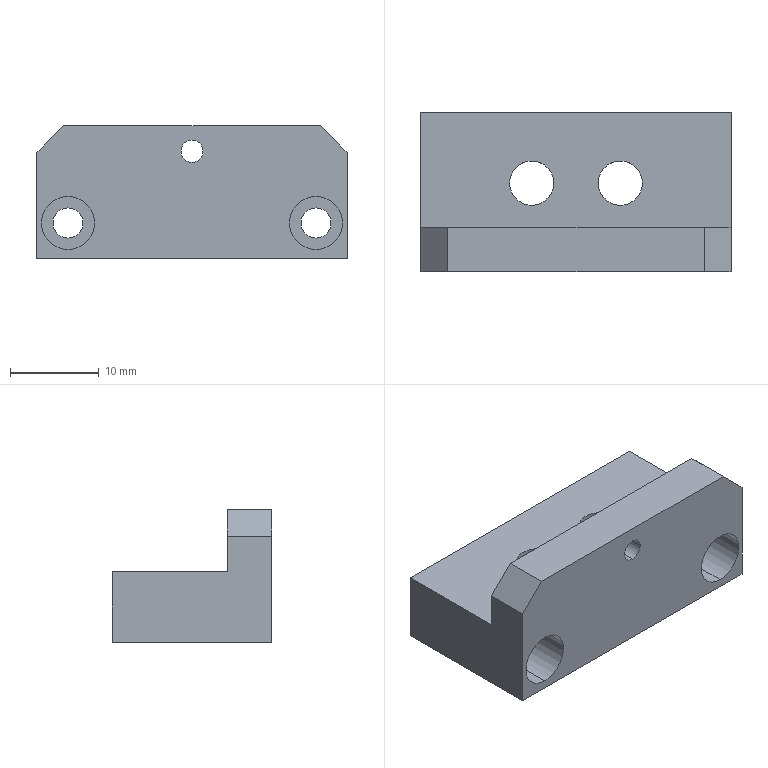Part | SolidWorks | features HoleWzd 4, Chamfer 1, Extrusion 1, ICE 1 | 1 solid | 34 faces | box 35 x 18 x 15 mm | volume 5316 mm3 | cylinder 18 | plane 12 | cone 4 | commonest cylinder face diameters 3 x4 3.4 x4 5 x4 6 x4 2.5 x2
STEP:
#1=CARTESIAN_POINT('',(-14.,-4.,-0.5));
#2=VERTEX_POINT('',#1);
#3=CARTESIAN_POINT('',(-14.,-4.,-6.5));
#4=VERTEX_POINT('',#3);
#5=CARTESIAN_POINT('',(-14.,-4.,-3.5));
#6=DIRECTION('',(0.,-1.,0.));
#7=DIRECTION('',(0.,0.,-1.));
#8=AXIS2_PLACEMENT_3D('',#5,#6,#7);
#9=CIRCLE('',#8,3.);
#10=EDGE_CURVE('',#2,#4,#9,.T.);
#11=ORIENTED_EDGE('',*,*,#10,.F.);
#12=CARTESIAN_POINT('',(-14.,-9.,-0.5));
#13=VERTEX_POINT('',#12);
#14=CARTESIAN_POINT('',(-14.,-9.,-0.5));
#15=DIRECTION('',(0.,-1.,0.));
#16=VECTOR('',#15,1000.);
#17=LINE('',#14,#16);
#18=EDGE_CURVE('',#2,#13,#17,.T.);
#19=ORIENTED_EDGE('',*,*,#18,.T.);
#20=CARTESIAN_POINT('',(-14.,-9.,-6.5));
#21=VERTEX_POINT('',#20);
#22=CARTESIAN_POINT('',(-14.,-9.,-3.5));
#23=DIRECTION('',(0.,-1.,0.));
#24=DIRECTION('',(0.,0.,-1.));
#25=AXIS2_PLACEMENT_3D('',#22,#23,#24);
#26=CIRCLE('',#25,3.);
#27=EDGE_CURVE('',#13,#21,#26,.T.);
#28=ORIENTED_EDGE('',*,*,#27,.T.);
#29=CARTESIAN_POINT('',(-14.,-9.,-6.5));
#30=DIRECTION('',(0.,-1.,0.));
#31=VECTOR('',#30,1000.);
#32=LINE('',#29,#31);
#33=EDGE_CURVE('',#4,#21,#32,.T.);
#34=ORIENTED_EDGE('',*,*,#33,.F.);
#35=EDGE_LOOP('',(#11,#19,#28,#34));
#36=FACE_OUTER_BOUND('',#35,.T.);
#37=CARTESIAN_POINT('',(-14.,-9.,-3.5));
#38=DIRECTION('',(0.,-1.,0.));
#39=DIRECTION('',(0.,0.,-1.));
#40=AXIS2_PLACEMENT_3D('',#37,#38,#39);
#41=CYLINDRICAL_SURFACE('',#40,3.);
#42=ADVANCED_FACE('',(#36),#41,.F.);
#43=CARTESIAN_POINT('',(-14.,9.,-1.8));
#44=VERTEX_POINT('',#43);
#45=CARTESIAN_POINT('',(-14.,9.,-5.2));
#46=VERTEX_POINT('',#45);
#47=CARTESIAN_POINT('',(-14.,9.,-3.5));
#48=DIRECTION('',(0.,-1.,0.));
#49=DIRECTION('',(0.,0.,-1.));
#50=AXIS2_PLACEMENT_3D('',#47,#48,#49);
#51=CIRCLE('',#50,1.7);
#52=EDGE_CURVE('',#44,#46,#51,.T.);
#53=ORIENTED_EDGE('',*,*,#52,.F.);
#54=CARTESIAN_POINT('',(-14.,-4.,-1.8));
#55=VERTEX_POINT('',#54);
#56=CARTESIAN_POINT('',(-14.,-9.,-1.8));
#57=DIRECTION('',(0.,-1.,0.));
#58=VECTOR('',#57,1000.);
#59=LINE('',#56,#58);
#60=EDGE_CURVE('',#44,#55,#59,.T.);
#61=ORIENTED_EDGE('',*,*,#60,.T.);
#62=CARTESIAN_POINT('',(-14.,-4.,-5.2));
#63=VERTEX_POINT('',#62);
#64=CARTESIAN_POINT('',(-14.,-4.,-3.5));
#65=DIRECTION('',(0.,-1.,0.));
#66=DIRECTION('',(0.,0.,-1.));
#67=AXIS2_PLACEMENT_3D('',#64,#65,#66);
#68=CIRCLE('',#67,1.7);
#69=EDGE_CURVE('',#55,#63,#68,.T.);
#70=ORIENTED_EDGE('',*,*,#69,.T.);
#71=CARTESIAN_POINT('',(-14.,-9.,-5.2));
#72=DIRECTION('',(0.,-1.,0.));
#73=VECTOR('',#72,1000.);
#74=LINE('',#71,#73);
#75=EDGE_CURVE('',#46,#63,#74,.T.);
#76=ORIENTED_EDGE('',*,*,#75,.F.);
#77=EDGE_LOOP('',(#53,#61,#70,#76));
#78=FACE_OUTER_BOUND('',#77,.T.);
#79=CARTESIAN_POINT('',(-14.,-9.,-3.5));
#80=DIRECTION('',(0.,-1.,0.));
#81=DIRECTION('',(0.,0.,-1.));
#82=AXIS2_PLACEMENT_3D('',#79,#80,#81);
#83=CYLINDRICAL_SURFACE('',#82,1.7);
#84=ADVANCED_FACE('',(#78),#83,.F.);
#85=CARTESIAN_POINT('',(14.,-4.,-0.5));
#86=VERTEX_POINT('',#85);
#87=CARTESIAN_POINT('',(14.,-4.,-6.5));
#88=VERTEX_POINT('',#87);
#89=CARTESIAN_POINT('',(14.,-4.,-3.5));
#90=DIRECTION('',(0.,-1.,0.));
#91=DIRECTION('',(0.,0.,-1.));
#92=AXIS2_PLACEMENT_3D('',#89,#90,#91);
#93=CIRCLE('',#92,3.);
#94=EDGE_CURVE('',#86,#88,#93,.T.);
#95=ORIENTED_EDGE('',*,*,#94,.F.);
#96=CARTESIAN_POINT('',(14.,-9.,-0.5));
#97=VERTEX_POINT('',#96);
#98=CARTESIAN_POINT('',(14.,-9.,-0.5));
#99=DIRECTION('',(0.,-1.,0.));
#100=VECTOR('',#99,1000.);
#101=LINE('',#98,#100);
#102=EDGE_CURVE('',#86,#97,#101,.T.);
#103=ORIENTED_EDGE('',*,*,#102,.T.);
#104=CARTESIAN_POINT('',(14.,-9.,-6.5));
#105=VERTEX_POINT('',#104);
#106=CARTESIAN_POINT('',(14.,-9.,-3.5));
#107=DIRECTION('',(0.,-1.,0.));
#108=DIRECTION('',(0.,0.,-1.));
#109=AXIS2_PLACEMENT_3D('',#106,#107,#108);
#110=CIRCLE('',#109,3.);
#111=EDGE_CURVE('',#97,#105,#110,.T.);
#112=ORIENTED_EDGE('',*,*,#111,.T.);
#113=CARTESIAN_POINT('',(14.,-9.,-6.5));
#114=DIRECTION('',(0.,-1.,0.));
#115=VECTOR('',#114,1000.);
#116=LINE('',#113,#115);
#117=EDGE_CURVE('',#88,#105,#116,.T.);
#118=ORIENTED_EDGE('',*,*,#117,.F.);
#119=EDGE_LOOP('',(#95,#103,#112,#118));
#120=FACE_OUTER_BOUND('',#119,.T.);
#121=CARTESIAN_POINT('',(14.,-9.,-3.5));
#122=DIRECTION('',(0.,-1.,0.));
#123=DIRECTION('',(0.,0.,-1.));
#124=AXIS2_PLACEMENT_3D('',#121,#122,#123);
#125=CYLINDRICAL_SURFACE('',#124,3.);
#126=ADVANCED_FACE('',(#120),#125,.F.);
#127=CARTESIAN_POINT('',(14.,9.,-1.8));
#128=VERTEX_POINT('',#127);
#129=CARTESIAN_POINT('',(14.,9.,-5.2));
#130=VERTEX_POINT('',#129);
#131=CARTESIAN_POINT('',(14.,9.,-3.5));
#132=DIRECTION('',(0.,-1.,0.));
#133=DIRECTION('',(0.,0.,-1.));
#134=AXIS2_PLACEMENT_3D('',#131,#132,#133);
#135=CIRCLE('',#134,1.7);
#136=EDGE_CURVE('',#128,#130,#135,.T.);
#137=ORIENTED_EDGE('',*,*,#136,.F.);
#138=CARTESIAN_POINT('',(14.,-4.,-1.8));
#139=VERTEX_POINT('',#138);
#140=CARTESIAN_POINT('',(14.,-9.,-1.8));
#141=DIRECTION('',(0.,-1.,0.));
#142=VECTOR('',#141,1000.);
#143=LINE('',#140,#142);
#144=EDGE_CURVE('',#128,#139,#143,.T.);
#145=ORIENTED_EDGE('',*,*,#144,.T.);
#146=CARTESIAN_POINT('',(14.,-4.,-5.2));
#147=VERTEX_POINT('',#146);
#148=CARTESIAN_POINT('',(14.,-4.,-3.5));
#149=DIRECTION('',(0.,-1.,0.));
#150=DIRECTION('',(0.,0.,-1.));
#151=AXIS2_PLACEMENT_3D('',#148,#149,#150);
#152=CIRCLE('',#151,1.7);
#153=EDGE_CURVE('',#139,#147,#152,.T.);
#154=ORIENTED_EDGE('',*,*,#153,.T.);
#155=CARTESIAN_POINT('',(14.,-9.,-5.2));
#156=DIRECTION('',(0.,-1.,0.));
#157=VECTOR('',#156,1000.);
#158=LINE('',#155,#157);
#159=EDGE_CURVE('',#130,#147,#158,.T.);
#160=ORIENTED_EDGE('',*,*,#159,.F.);
#161=EDGE_LOOP('',(#137,#145,#154,#160));
#162=FACE_OUTER_BOUND('',#161,.T.);
#163=CARTESIAN_POINT('',(14.,-9.,-3.5));
#164=DIRECTION('',(0.,-1.,0.));
#165=DIRECTION('',(0.,0.,-1.));
#166=AXIS2_PLACEMENT_3D('',#163,#164,#165);
#167=CYLINDRICAL_SURFACE('',#166,1.7);
#168=ADVANCED_FACE('',(#162),#167,.F.);
#169=CARTESIAN_POINT('',(0.,-4.,5.85));
#170=VERTEX_POINT('',#169);
#171=CARTESIAN_POINT('',(0.,-4.,3.35));
#172=VERTEX_POINT('',#171);
#173=CARTESIAN_POINT('',(0.,-4.,4.6));
#174=DIRECTION('',(0.,-1.,0.));
#175=DIRECTION('',(1.,0.,0.));
#176=AXIS2_PLACEMENT_3D('',#173,#174,#175);
#177=CIRCLE('',#176,1.25);
#178=EDGE_CURVE('',#170,#172,#177,.T.);
#179=ORIENTED_EDGE('',*,*,#178,.F.);
#180=CARTESIAN_POINT('',(0.,-9.,5.85));
#181=VERTEX_POINT('',#180);
#182=CARTESIAN_POINT('',(0.,-9.,5.85));
#183=DIRECTION('',(0.,-1.,0.));
#184=VECTOR('',#183,1000.);
#185=LINE('',#182,#184);
#186=EDGE_CURVE('',#170,#181,#185,.T.);
#187=ORIENTED_EDGE('',*,*,#186,.T.);
#188=CARTESIAN_POINT('',(0.,-9.,3.35));
#189=VERTEX_POINT('',#188);
#190=CARTESIAN_POINT('',(0.,-9.,4.6));
#191=DIRECTION('',(0.,-1.,0.));
#192=DIRECTION('',(0.,0.,-1.));
#193=AXIS2_PLACEMENT_3D('',#190,#191,#192);
#194=CIRCLE('',#193,1.25);
#195=EDGE_CURVE('',#181,#189,#194,.T.);
#196=ORIENTED_EDGE('',*,*,#195,.T.);
#197=CARTESIAN_POINT('',(0.,-9.,3.35));
#198=DIRECTION('',(0.,-1.,0.));
#199=VECTOR('',#198,1000.);
#200=LINE('',#197,#199);
#201=EDGE_CURVE('',#172,#189,#200,.T.);
#202=ORIENTED_EDGE('',*,*,#201,.F.);
#203=EDGE_LOOP('',(#179,#187,#196,#202));
#204=FACE_OUTER_BOUND('',#203,.T.);
#205=CARTESIAN_POINT('',(0.,-9.,4.6));
#206=DIRECTION('',(0.,-1.,0.));
#207=DIRECTION('',(0.,0.,-1.));
#208=AXIS2_PLACEMENT_3D('',#205,#206,#207);
#209=CYLINDRICAL_SURFACE('',#208,1.25);
#210=ADVANCED_FACE('',(#204),#209,.F.);
#211=CARTESIAN_POINT('',(10.2,-7.,3.1));
#212=VERTEX_POINT('',#211);
#213=CARTESIAN_POINT('',(10.2,-7.,6.1));
#214=VERTEX_POINT('',#213);
#215=CARTESIAN_POINT('',(10.2,-7.,4.6));
#216=DIRECTION('',(0.,1.,0.));
#217=DIRECTION('',(0.,0.,1.));
#218=AXIS2_PLACEMENT_3D('',#215,#216,#217);
#219=CIRCLE('',#218,1.5);
#220=EDGE_CURVE('',#212,#214,#219,.T.);
#221=ORIENTED_EDGE('',*,*,#220,.F.);
#222=CARTESIAN_POINT('',(10.2,-4.,3.1));
#223=VERTEX_POINT('',#222);
#224=CARTESIAN_POINT('',(10.2,-4.,3.1));
#225=DIRECTION('',(0.,1.,0.));
#226=VECTOR('',#225,1000.);
#227=LINE('',#224,#226);
#228=EDGE_CURVE('',#212,#223,#227,.T.);
#229=ORIENTED_EDGE('',*,*,#228,.T.);
#230=CARTESIAN_POINT('',(10.2,-4.,6.1));
#231=VERTEX_POINT('',#230);
#232=CARTESIAN_POINT('',(10.2,-4.,4.6));
#233=DIRECTION('',(0.,1.,0.));
#234=DIRECTION('',(0.,0.,1.));
#235=AXIS2_PLACEMENT_3D('',#232,#233,#234);
#236=CIRCLE('',#235,1.5);
#237=EDGE_CURVE('',#223,#231,#236,.T.);
#238=ORIENTED_EDGE('',*,*,#237,.T.);
#239=CARTESIAN_POINT('',(10.2,-4.,6.1));
#240=DIRECTION('',(0.,1.,0.));
#241=VECTOR('',#240,1000.);
#242=LINE('',#239,#241);
#243=EDGE_CURVE('',#214,#231,#242,.T.);
#244=ORIENTED_EDGE('',*,*,#243,.F.);
#245=EDGE_LOOP('',(#221,#229,#238,#244));
#246=FACE_OUTER_BOUND('',#245,.T.);
#247=CARTESIAN_POINT('',(10.2,-4.,4.6));
#248=DIRECTION('',(0.,1.,0.));
#249=DIRECTION('',(0.,0.,1.));
#250=AXIS2_PLACEMENT_3D('',#247,#248,#249);
#251=CYLINDRICAL_SURFACE('',#250,1.5);
#252=ADVANCED_FACE('',(#246),#251,.F.);
#253=CARTESIAN_POINT('',(10.2,-7.901,4.6));
#254=VERTEX_POINT('',#253);
#255=CARTESIAN_POINT('',(10.2,-7.,6.1));
#256=DIRECTION('',(0.,0.515,0.8572));
#257=VECTOR('',#256,1000.);
#258=LINE('',#255,#257);
#259=EDGE_CURVE('',#254,#214,#258,.T.);
#260=ORIENTED_EDGE('',*,*,#259,.F.);
#261=CARTESIAN_POINT('',(10.2,-7.,3.1));
#262=DIRECTION('',(0.,0.515,-0.8572));
#263=VECTOR('',#262,1000.);
#264=LINE('',#261,#263);
#265=EDGE_CURVE('',#254,#212,#264,.T.);
#266=ORIENTED_EDGE('',*,*,#265,.T.);
#267=ORIENTED_EDGE('',*,*,#220,.T.);
#268=EDGE_LOOP('',(#260,#266,#267));
#269=FACE_OUTER_BOUND('',#268,.T.);
#270=CARTESIAN_POINT('',(10.2,-7.,4.6));
#271=DIRECTION('',(0.,1.,0.));
#272=DIRECTION('',(0.,0.,1.));
#273=AXIS2_PLACEMENT_3D('',#270,#271,#272);
#274=CONICAL_SURFACE('',#273,1.5,1.03);
#275=ADVANCED_FACE('',(#269),#274,.F.);
#276=CARTESIAN_POINT('',(-10.2,-7.,3.1));
#277=VERTEX_POINT('',#276);
#278=CARTESIAN_POINT('',(-10.2,-7.,6.1));
#279=VERTEX_POINT('',#278);
#280=CARTESIAN_POINT('',(-10.2,-7.,4.6));
#281=DIRECTION('',(0.,1.,0.));
#282=DIRECTION('',(0.,0.,1.));
#283=AXIS2_PLACEMENT_3D('',#280,#281,#282);
#284=CIRCLE('',#283,1.5);
#285=EDGE_CURVE('',#277,#279,#284,.T.);
#286=ORIENTED_EDGE('',*,*,#285,.F.);
#287=CARTESIAN_POINT('',(-10.2,-4.,3.1));
#288=VERTEX_POINT('',#287);
#289=CARTESIAN_POINT('',(-10.2,-4.,3.1));
#290=DIRECTION('',(0.,1.,0.));
#291=VECTOR('',#290,1000.);
#292=LINE('',#289,#291);
#293=EDGE_CURVE('',#277,#288,#292,.T.);
#294=ORIENTED_EDGE('',*,*,#293,.T.);
#295=CARTESIAN_POINT('',(-10.2,-4.,6.1));
#296=VERTEX_POINT('',#295);
#297=CARTESIAN_POINT('',(-10.2,-4.,4.6));
#298=DIRECTION('',(0.,1.,0.));
#299=DIRECTION('',(0.,0.,1.));
#300=AXIS2_PLACEMENT_3D('',#297,#298,#299);
#301=CIRCLE('',#300,1.5);
#302=EDGE_CURVE('',#288,#296,#301,.T.);
#303=ORIENTED_EDGE('',*,*,#302,.T.);
#304=CARTESIAN_POINT('',(-10.2,-4.,6.1));
#305=DIRECTION('',(0.,1.,0.));
#306=VECTOR('',#305,1000.);
#307=LINE('',#304,#306);
#308=EDGE_CURVE('',#279,#296,#307,.T.);
#309=ORIENTED_EDGE('',*,*,#308,.F.);
#310=EDGE_LOOP('',(#286,#294,#303,#309));
#311=FACE_OUTER_BOUND('',#310,.T.);
#312=CARTESIAN_POINT('',(-10.2,-4.,4.6));
#313=DIRECTION('',(0.,1.,0.));
#314=DIRECTION('',(0.,0.,1.));
#315=AXIS2_PLACEMENT_3D('',#312,#313,#314);
#316=CYLINDRICAL_SURFACE('',#315,1.5);
#317=ADVANCED_FACE('',(#311),#316,.F.);
#318=CARTESIAN_POINT('',(-10.2,-7.901,4.6));
#319=VERTEX_POINT('',#318);
#320=CARTESIAN_POINT('',(-10.2,-7.,6.1));
#321=DIRECTION('',(0.,0.515,0.8572));
#322=VECTOR('',#321,1000.);
#323=LINE('',#320,#322);
#324=EDGE_CURVE('',#319,#279,#323,.T.);
#325=ORIENTED_EDGE('',*,*,#324,.F.);
#326=CARTESIAN_POINT('',(-10.2,-7.,3.1));
#327=DIRECTION('',(0.,0.515,-0.8572));
#328=VECTOR('',#327,1000.);
#329=LINE('',#326,#328);
#330=EDGE_CURVE('',#319,#277,#329,.T.);
#331=ORIENTED_EDGE('',*,*,#330,.T.);
#332=ORIENTED_EDGE('',*,*,#285,.T.);
#333=EDGE_LOOP('',(#325,#331,#332));
#334=FACE_OUTER_BOUND('',#333,.T.);
#335=CARTESIAN_POINT('',(-10.2,-7.,4.6));
#336=DIRECTION('',(0.,1.,0.));
#337=DIRECTION('',(0.,0.,1.));
#338=AXIS2_PLACEMENT_3D('',#335,#336,#337);
#339=CONICAL_SURFACE('',#338,1.5,1.03);
#340=ADVANCED_FACE('',(#334),#339,.F.);
#341=CARTESIAN_POINT('',(-7.5,1.,-7.5));
#342=VERTEX_POINT('',#341);
#343=CARTESIAN_POINT('',(-2.5,1.,-7.5));
#344=VERTEX_POINT('',#343);
#345=CARTESIAN_POINT('',(-5.,1.,-7.5));
#346=DIRECTION('',(0.,0.,1.));
#347=DIRECTION('',(1.,0.,0.));
#348=AXIS2_PLACEMENT_3D('',#345,#346,#347);
#349=CIRCLE('',#348,2.5);
#350=EDGE_CURVE('',#342,#344,#349,.T.);
#351=ORIENTED_EDGE('',*,*,#350,.F.);
#352=CARTESIAN_POINT('',(-7.5,1.,0.5));
#353=VERTEX_POINT('',#352);
#354=CARTESIAN_POINT('',(-7.5,1.,0.5));
#355=DIRECTION('',(0.,0.,1.));
#356=VECTOR('',#355,1000.);
#357=LINE('',#354,#356);
#358=EDGE_CURVE('',#342,#353,#357,.T.);
#359=ORIENTED_EDGE('',*,*,#358,.T.);
#360=CARTESIAN_POINT('',(-2.5,1.,0.5));
#361=VERTEX_POINT('',#360);
#362=CARTESIAN_POINT('',(-5.,1.,0.5));
#363=DIRECTION('',(0.,0.,1.));
#364=DIRECTION('',(1.,0.,0.));
#365=AXIS2_PLACEMENT_3D('',#362,#363,#364);
#366=CIRCLE('',#365,2.5);
#367=EDGE_CURVE('',#353,#361,#366,.T.);
#368=ORIENTED_EDGE('',*,*,#367,.T.);
#369=CARTESIAN_POINT('',(-2.5,1.,0.5));
#370=DIRECTION('',(0.,0.,1.));
#371=VECTOR('',#370,1000.);
#372=LINE('',#369,#371);
#373=EDGE_CURVE('',#344,#361,#372,.T.);
#374=ORIENTED_EDGE('',*,*,#373,.F.);
#375=EDGE_LOOP('',(#351,#359,#368,#374));
#376=FACE_OUTER_BOUND('',#375,.T.);
#377=CARTESIAN_POINT('',(-5.,1.,0.5));
#378=DIRECTION('',(0.,0.,1.));
#379=DIRECTION('',(1.,0.,0.));
#380=AXIS2_PLACEMENT_3D('',#377,#378,#379);
#381=CYLINDRICAL_SURFACE('',#380,2.5);
#382=ADVANCED_FACE('',(#376),#381,.F.);
#383=CARTESIAN_POINT('',(2.5,1.,-7.5));
#384=VERTEX_POINT('',#383);
#385=CARTESIAN_POINT('',(7.5,1.,-7.5));
#386=VERTEX_POINT('',#385);
#387=CARTESIAN_POINT('',(5.,1.,-7.5));
#388=DIRECTION('',(0.,0.,1.));
#389=DIRECTION('',(1.,0.,0.));
#390=AXIS2_PLACEMENT_3D('',#387,#388,#389);
#391=CIRCLE('',#390,2.5);
#392=EDGE_CURVE('',#384,#386,#391,.T.);
#393=ORIENTED_EDGE('',*,*,#392,.F.);
#394=CARTESIAN_POINT('',(2.5,1.,0.5));
#395=VERTEX_POINT('',#394);
#396=CARTESIAN_POINT('',(2.5,1.,0.5));
#397=DIRECTION('',(0.,0.,1.));
#398=VECTOR('',#397,1000.);
#399=LINE('',#396,#398);
#400=EDGE_CURVE('',#384,#395,#399,.T.);
#401=ORIENTED_EDGE('',*,*,#400,.T.);
#402=CARTESIAN_POINT('',(7.5,1.,0.5));
#403=VERTEX_POINT('',#402);
#404=CARTESIAN_POINT('',(5.,1.,0.5));
#405=DIRECTION('',(0.,0.,1.));
#406=DIRECTION('',(1.,0.,0.));
#407=AXIS2_PLACEMENT_3D('',#404,#405,#406);
#408=CIRCLE('',#407,2.5);
#409=EDGE_CURVE('',#395,#403,#408,.T.);
#410=ORIENTED_EDGE('',*,*,#409,.T.);
#411=CARTESIAN_POINT('',(7.5,1.,0.5));
#412=DIRECTION('',(0.,0.,1.));
#413=VECTOR('',#412,1000.);
#414=LINE('',#411,#413);
#415=EDGE_CURVE('',#386,#403,#414,.T.);
#416=ORIENTED_EDGE('',*,*,#415,.F.);
#417=EDGE_LOOP('',(#393,#401,#410,#416));
#418=FACE_OUTER_BOUND('',#417,.T.);
#419=CARTESIAN_POINT('',(5.,1.,0.5));
#420=DIRECTION('',(0.,0.,1.));
#421=DIRECTION('',(1.,0.,0.));
#422=AXIS2_PLACEMENT_3D('',#419,#420,#421);
#423=CYLINDRICAL_SURFACE('',#422,2.5);
#424=ADVANCED_FACE('',(#418),#423,.F.);
#425=CARTESIAN_POINT('',(17.5,-4.,4.5));
#426=VERTEX_POINT('',#425);
#427=CARTESIAN_POINT('',(17.5,-4.,0.5));
#428=VERTEX_POINT('',#427);
#429=CARTESIAN_POINT('',(17.5,-4.,7.5));
#430=DIRECTION('',(0.,0.,-1.));
#431=VECTOR('',#430,1000.);
#432=LINE('',#429,#431);
#433=EDGE_CURVE('',#426,#428,#432,.T.);
#434=ORIENTED_EDGE('',*,*,#433,.F.);
#435=CARTESIAN_POINT('',(17.5,-9.,4.5));
#436=VERTEX_POINT('',#435);
#437=CARTESIAN_POINT('',(17.5,-9.,4.5));
#438=DIRECTION('',(0.,-1.,0.));
#439=VECTOR('',#438,1000.);
#440=LINE('',#437,#439);
#441=EDGE_CURVE('',#426,#436,#440,.T.);
#442=ORIENTED_EDGE('',*,*,#441,.T.);
#443=CARTESIAN_POINT('',(17.5,-9.,-7.5));
#444=VERTEX_POINT('',#443);
#445=CARTESIAN_POINT('',(17.5,-9.,7.5));
#446=DIRECTION('',(0.,0.,-1.));
#447=VECTOR('',#446,1000.);
#448=LINE('',#445,#447);
#449=EDGE_CURVE('',#436,#444,#448,.T.);
#450=ORIENTED_EDGE('',*,*,#449,.T.);
#451=CARTESIAN_POINT('',(17.5,9.,-7.5));
#452=VERTEX_POINT('',#451);
#453=CARTESIAN_POINT('',(17.5,9.,-7.5));
#454=DIRECTION('',(0.,1.,0.));
#455=VECTOR('',#454,1000.);
#456=LINE('',#453,#455);
#457=EDGE_CURVE('',#444,#452,#456,.T.);
#458=ORIENTED_EDGE('',*,*,#457,.T.);
#459=CARTESIAN_POINT('',(17.5,9.,0.5));
#460=VERTEX_POINT('',#459);
#461=CARTESIAN_POINT('',(17.5,9.,7.5));
#462=DIRECTION('',(0.,0.,-1.));
#463=VECTOR('',#462,1000.);
#464=LINE('',#461,#463);
#465=EDGE_CURVE('',#460,#452,#464,.T.);
#466=ORIENTED_EDGE('',*,*,#465,.F.);
#467=CARTESIAN_POINT('',(17.5,9.,0.5));
#468=DIRECTION('',(0.,1.,0.));
#469=VECTOR('',#468,1000.);
#470=LINE('',#467,#469);
#471=EDGE_CURVE('',#428,#460,#470,.T.);
#472=ORIENTED_EDGE('',*,*,#471,.F.);
#473=EDGE_LOOP('',(#434,#442,#450,#458,#466,#472));
#474=FACE_OUTER_BOUND('',#473,.T.);
#475=CARTESIAN_POINT('',(17.5,9.,7.5));
#476=DIRECTION('',(-1.,0.,0.));
#477=DIRECTION('',(0.,-1.,0.));
#478=AXIS2_PLACEMENT_3D('',#475,#476,#477);
#479=PLANE('',#478);
#480=ADVANCED_FACE('',(#474),#479,.F.);
#481=CARTESIAN_POINT('',(-14.,9.,-3.5));
#482=DIRECTION('',(0.,-1.,0.));
#483=DIRECTION('',(0.,0.,-1.));
#484=AXIS2_PLACEMENT_3D('',#481,#482,#483);
#485=CIRCLE('',#484,1.7);
#486=EDGE_CURVE('',#46,#44,#485,.T.);
#487=ORIENTED_EDGE('',*,*,#486,.T.);
#488=ORIENTED_EDGE('',*,*,#52,.T.);
#489=EDGE_LOOP('',(#487,#488));
#490=FACE_BOUND('',#489,.T.);
#491=CARTESIAN_POINT('',(14.,9.,-3.5));
#492=DIRECTION('',(0.,-1.,0.));
#493=DIRECTION('',(0.,0.,-1.));
#494=AXIS2_PLACEMENT_3D('',#491,#492,#493);
#495=CIRCLE('',#494,1.7);
#496=EDGE_CURVE('',#130,#128,#495,.T.);
#497=ORIENTED_EDGE('',*,*,#496,.T.);
#498=ORIENTED_EDGE('',*,*,#136,.T.);
#499=EDGE_LOOP('',(#497,#498));
#500=FACE_BOUND('',#499,.T.);
#501=CARTESIAN_POINT('',(-17.5,9.,0.5));
#502=VERTEX_POINT('',#501);
#503=CARTESIAN_POINT('',(-17.5,9.,-7.5));
#504=VERTEX_POINT('',#503);
#505=CARTESIAN_POINT('',(-17.5,9.,7.5));
#506=DIRECTION('',(0.,0.,-1.));
#507=VECTOR('',#506,1000.);
#508=LINE('',#505,#507);
#509=EDGE_CURVE('',#502,#504,#508,.T.);
#510=ORIENTED_EDGE('',*,*,#509,.F.);
#511=CARTESIAN_POINT('',(-17.5,9.,0.5));
#512=DIRECTION('',(1.,0.,0.));
#513=VECTOR('',#512,1000.);
#514=LINE('',#511,#513);
#515=EDGE_CURVE('',#502,#460,#514,.T.);
#516=ORIENTED_EDGE('',*,*,#515,.T.);
#517=ORIENTED_EDGE('',*,*,#465,.T.);
#518=CARTESIAN_POINT('',(-17.5,9.,-7.5));
#519=DIRECTION('',(-1.,0.,0.));
#520=VECTOR('',#519,1000.);
#521=LINE('',#518,#520);
#522=EDGE_CURVE('',#452,#504,#521,.T.);
#523=ORIENTED_EDGE('',*,*,#522,.T.);
#524=EDGE_LOOP('',(#510,#516,#517,#523));
#525=FACE_OUTER_BOUND('',#524,.T.);
#526=CARTESIAN_POINT('',(-17.5,9.,7.5));
#527=DIRECTION('',(0.,-1.,0.));
#528=DIRECTION('',(0.,0.,-1.));
#529=AXIS2_PLACEMENT_3D('',#526,#527,#528);
#530=PLANE('',#529);
#531=ADVANCED_FACE('',(#490,#500,#525),#530,.F.);
#532=CARTESIAN_POINT('',(-17.5,-9.,4.5));
#533=VERTEX_POINT('',#532);
#534=CARTESIAN_POINT('',(-17.5,-9.,-7.5));
#535=VERTEX_POINT('',#534);
#536=CARTESIAN_POINT('',(-17.5,-9.,7.5));
#537=DIRECTION('',(0.,0.,-1.));
#538=VECTOR('',#537,1000.);
#539=LINE('',#536,#538);
#540=EDGE_CURVE('',#533,#535,#539,.T.);
#541=ORIENTED_EDGE('',*,*,#540,.F.);
#542=CARTESIAN_POINT('',(-17.5,-4.,4.5));
#543=VERTEX_POINT('',#542);
#544=CARTESIAN_POINT('',(-17.5,-4.,4.5));
#545=DIRECTION('',(0.,1.,0.));
#546=VECTOR('',#545,1000.);
#547=LINE('',#544,#546);
#548=EDGE_CURVE('',#533,#543,#547,.T.);
#549=ORIENTED_EDGE('',*,*,#548,.T.);
#550=CARTESIAN_POINT('',(-17.5,-4.,0.5));
#551=VERTEX_POINT('',#550);
#552=CARTESIAN_POINT('',(-17.5,-4.,7.5));
#553=DIRECTION('',(0.,0.,-1.));
#554=VECTOR('',#553,1000.);
#555=LINE('',#552,#554);
#556=EDGE_CURVE('',#543,#551,#555,.T.);
#557=ORIENTED_EDGE('',*,*,#556,.T.);
#558=CARTESIAN_POINT('',(-17.5,9.,0.5));
#559=DIRECTION('',(0.,1.,0.));
#560=VECTOR('',#559,1000.);
#561=LINE('',#558,#560);
#562=EDGE_CURVE('',#551,#502,#561,.T.);
#563=ORIENTED_EDGE('',*,*,#562,.T.);
#564=ORIENTED_EDGE('',*,*,#509,.T.);
#565=CARTESIAN_POINT('',(-17.5,9.,-7.5));
#566=DIRECTION('',(0.,-1.,0.));
#567=VECTOR('',#566,1000.);
#568=LINE('',#565,#567);
#569=EDGE_CURVE('',#504,#535,#568,.T.);
#570=ORIENTED_EDGE('',*,*,#569,.T.);
#571=EDGE_LOOP('',(#541,#549,#557,#563,#564,#570));
#572=FACE_OUTER_BOUND('',#571,.T.);
#573=CARTESIAN_POINT('',(-17.5,9.,7.5));
#574=DIRECTION('',(1.,0.,0.));
#575=DIRECTION('',(0.,1.,0.));
#576=AXIS2_PLACEMENT_3D('',#573,#574,#575);
#577=PLANE('',#576);
#578=ADVANCED_FACE('',(#572),#577,.F.);
#579=CARTESIAN_POINT('',(-14.,-9.,-3.5));
#580=DIRECTION('',(0.,-1.,0.));
#581=DIRECTION('',(0.,0.,-1.));
#582=AXIS2_PLACEMENT_3D('',#579,#580,#581);
#583=CIRCLE('',#582,3.);
#584=EDGE_CURVE('',#21,#13,#583,.T.);
#585=ORIENTED_EDGE('',*,*,#584,.F.);
#586=ORIENTED_EDGE('',*,*,#27,.F.);
#587=EDGE_LOOP('',(#585,#586));
#588=FACE_BOUND('',#587,.T.);
#589=CARTESIAN_POINT('',(14.,-9.,-3.5));
#590=DIRECTION('',(0.,-1.,0.));
#591=DIRECTION('',(0.,0.,-1.));
#592=AXIS2_PLACEMENT_3D('',#589,#590,#591);
#593=CIRCLE('',#592,3.);
#594=EDGE_CURVE('',#105,#97,#593,.T.);
#595=ORIENTED_EDGE('',*,*,#594,.F.);
#596=ORIENTED_EDGE('',*,*,#111,.F.);
#597=EDGE_LOOP('',(#595,#596));
#598=FACE_BOUND('',#597,.T.);
#599=CARTESIAN_POINT('',(0.,-9.,4.6));
#600=DIRECTION('',(0.,-1.,0.));
#601=DIRECTION('',(0.,0.,-1.));
#602=AXIS2_PLACEMENT_3D('',#599,#600,#601);
#603=CIRCLE('',#602,1.25);
#604=EDGE_CURVE('',#189,#181,#603,.T.);
#605=ORIENTED_EDGE('',*,*,#604,.F.);
#606=ORIENTED_EDGE('',*,*,#195,.F.);
#607=EDGE_LOOP('',(#605,#606));
#608=FACE_BOUND('',#607,.T.);
#609=CARTESIAN_POINT('',(-14.5,-9.,7.5));
#610=VERTEX_POINT('',#609);
#611=CARTESIAN_POINT('',(14.5,-9.,7.5));
#612=VERTEX_POINT('',#611);
#613=CARTESIAN_POINT('',(-17.5,-9.,7.5));
#614=DIRECTION('',(1.,0.,0.));
#615=VECTOR('',#614,1000.);
#616=LINE('',#613,#615);
#617=EDGE_CURVE('',#610,#612,#616,.T.);
#618=ORIENTED_EDGE('',*,*,#617,.F.);
#619=CARTESIAN_POINT('',(-14.5,-9.,7.5));
#620=DIRECTION('',(-0.7071,0.,-0.7071));
#621=VECTOR('',#620,1000.);
#622=LINE('',#619,#621);
#623=EDGE_CURVE('',#610,#533,#622,.T.);
#624=ORIENTED_EDGE('',*,*,#623,.T.);
#625=ORIENTED_EDGE('',*,*,#540,.T.);
#626=CARTESIAN_POINT('',(-17.5,-9.,-7.5));
#627=DIRECTION('',(1.,0.,0.));
#628=VECTOR('',#627,1000.);
#629=LINE('',#626,#628);
#630=EDGE_CURVE('',#535,#444,#629,.T.);
#631=ORIENTED_EDGE('',*,*,#630,.T.);
#632=ORIENTED_EDGE('',*,*,#449,.F.);
#633=CARTESIAN_POINT('',(14.5,-9.,7.5));
#634=DIRECTION('',(-0.7071,0.,0.7071));
#635=VECTOR('',#634,1000.);
#636=LINE('',#633,#635);
#637=EDGE_CURVE('',#436,#612,#636,.T.);
#638=ORIENTED_EDGE('',*,*,#637,.T.);
#639=EDGE_LOOP('',(#618,#624,#625,#631,#632,#638));
#640=FACE_OUTER_BOUND('',#639,.T.);
#641=CARTESIAN_POINT('',(-17.5,-9.,7.5));
#642=DIRECTION('',(0.,1.,0.));
#643=DIRECTION('',(0.,0.,1.));
#644=AXIS2_PLACEMENT_3D('',#641,#642,#643);
#645=PLANE('',#644);
#646=ADVANCED_FACE('',(#588,#598,#608,#640),#645,.F.);
#647=CARTESIAN_POINT('',(-14.5,-4.,7.5));
#648=VERTEX_POINT('',#647);
#649=CARTESIAN_POINT('',(14.5,-4.,7.5));
#650=VERTEX_POINT('',#649);
#651=CARTESIAN_POINT('',(-17.5,-4.,7.5));
#652=DIRECTION('',(1.,0.,0.));
#653=VECTOR('',#652,1000.);
#654=LINE('',#651,#653);
#655=EDGE_CURVE('',#648,#650,#654,.T.);
#656=ORIENTED_EDGE('',*,*,#655,.F.);
#657=CARTESIAN_POINT('',(-14.5,-9.,7.5));
#658=DIRECTION('',(0.,-1.,0.));
#659=VECTOR('',#658,1000.);
#660=LINE('',#657,#659);
#661=EDGE_CURVE('',#648,#610,#660,.T.);
#662=ORIENTED_EDGE('',*,*,#661,.T.);
#663=ORIENTED_EDGE('',*,*,#617,.T.);
#664=CARTESIAN_POINT('',(14.5,-4.,7.5));
#665=DIRECTION('',(0.,1.,0.));
#666=VECTOR('',#665,1000.);
#667=LINE('',#664,#666);
#668=EDGE_CURVE('',#612,#650,#667,.T.);
#669=ORIENTED_EDGE('',*,*,#668,.T.);
#670=EDGE_LOOP('',(#656,#662,#663,#669));
#671=FACE_OUTER_BOUND('',#670,.T.);
#672=CARTESIAN_POINT('',(0.,0.,7.5));
#673=DIRECTION('',(0.,0.,1.));
#674=DIRECTION('',(1.,0.,0.));
#675=AXIS2_PLACEMENT_3D('',#672,#673,#674);
#676=PLANE('',#675);
#677=ADVANCED_FACE('',(#671),#676,.T.);
#678=CARTESIAN_POINT('',(-5.,1.,-7.5));
#679=DIRECTION('',(0.,0.,1.));
#680=DIRECTION('',(1.,0.,0.));
#681=AXIS2_PLACEMENT_3D('',#678,#679,#680);
#682=CIRCLE('',#681,2.5);
#683=EDGE_CURVE('',#344,#342,#682,.T.);
#684=ORIENTED_EDGE('',*,*,#683,.T.);
#685=ORIENTED_EDGE('',*,*,#350,.T.);
#686=EDGE_LOOP('',(#684,#685));
#687=FACE_BOUND('',#686,.T.);
#688=CARTESIAN_POINT('',(5.,1.,-7.5));
#689=DIRECTION('',(0.,0.,1.));
#690=DIRECTION('',(1.,0.,0.));
#691=AXIS2_PLACEMENT_3D('',#688,#689,#690);
#692=CIRCLE('',#691,2.5);
#693=EDGE_CURVE('',#386,#384,#692,.T.);
#694=ORIENTED_EDGE('',*,*,#693,.T.);
#695=ORIENTED_EDGE('',*,*,#392,.T.);
#696=EDGE_LOOP('',(#694,#695));
#697=FACE_BOUND('',#696,.T.);
#698=ORIENTED_EDGE('',*,*,#457,.F.);
#699=ORIENTED_EDGE('',*,*,#630,.F.);
#700=ORIENTED_EDGE('',*,*,#569,.F.);
#701=ORIENTED_EDGE('',*,*,#522,.F.);
#702=EDGE_LOOP('',(#698,#699,#700,#701));
#703=FACE_OUTER_BOUND('',#702,.T.);
#704=CARTESIAN_POINT('',(0.,0.,-7.5));
#705=DIRECTION('',(0.,0.,1.));
#706=DIRECTION('',(1.,0.,0.));
#707=AXIS2_PLACEMENT_3D('',#704,#705,#706);
#708=PLANE('',#707);
#709=ADVANCED_FACE('',(#687,#697,#703),#708,.F.);
#710=CARTESIAN_POINT('',(-5.,1.,0.5));
#711=DIRECTION('',(0.,0.,1.));
#712=DIRECTION('',(1.,0.,0.));
#713=AXIS2_PLACEMENT_3D('',#710,#711,#712);
#714=CIRCLE('',#713,2.5);
#715=EDGE_CURVE('',#361,#353,#714,.T.);
#716=ORIENTED_EDGE('',*,*,#715,.F.);
#717=ORIENTED_EDGE('',*,*,#367,.F.);
#718=EDGE_LOOP('',(#716,#717));
#719=FACE_BOUND('',#718,.T.);
#720=CARTESIAN_POINT('',(5.,1.,0.5));
#721=DIRECTION('',(0.,0.,1.));
#722=DIRECTION('',(1.,0.,0.));
#723=AXIS2_PLACEMENT_3D('',#720,#721,#722);
#724=CIRCLE('',#723,2.5);
#725=EDGE_CURVE('',#403,#395,#724,.T.);
#726=ORIENTED_EDGE('',*,*,#725,.F.);
#727=ORIENTED_EDGE('',*,*,#409,.F.);
#728=EDGE_LOOP('',(#726,#727));
#729=FACE_BOUND('',#728,.T.);
#730=ORIENTED_EDGE('',*,*,#471,.T.);
#731=ORIENTED_EDGE('',*,*,#515,.F.);
#732=ORIENTED_EDGE('',*,*,#562,.F.);
#733=CARTESIAN_POINT('',(-17.5,-4.,0.5));
#734=DIRECTION('',(1.,0.,0.));
#735=VECTOR('',#734,1000.);
#736=LINE('',#733,#735);
#737=EDGE_CURVE('',#551,#428,#736,.T.);
#738=ORIENTED_EDGE('',*,*,#737,.T.);
#739=EDGE_LOOP('',(#730,#731,#732,#738));
#740=FACE_OUTER_BOUND('',#739,.T.);
#741=CARTESIAN_POINT('',(-17.5,9.,0.5));
#742=DIRECTION('',(0.,0.,-1.));
#743=DIRECTION('',(0.,1.,0.));
#744=AXIS2_PLACEMENT_3D('',#741,#742,#743);
#745=PLANE('',#744);
#746=ADVANCED_FACE('',(#719,#729,#740),#745,.F.);
#747=CARTESIAN_POINT('',(0.,-4.,4.6));
#748=DIRECTION('',(0.,-1.,0.));
#749=DIRECTION('',(1.,0.,0.));
#750=AXIS2_PLACEMENT_3D('',#747,#748,#749);
#751=CIRCLE('',#750,1.25);
#752=EDGE_CURVE('',#172,#170,#751,.T.);
#753=ORIENTED_EDGE('',*,*,#752,.T.);
#754=ORIENTED_EDGE('',*,*,#178,.T.);
#755=EDGE_LOOP('',(#753,#754));
#756=FACE_BOUND('',#755,.T.);
#757=CARTESIAN_POINT('',(10.2,-4.,4.6));
#758=DIRECTION('',(0.,1.,0.));
#759=DIRECTION('',(0.,0.,1.));
#760=AXIS2_PLACEMENT_3D('',#757,#758,#759);
#761=CIRCLE('',#760,1.5);
#762=EDGE_CURVE('',#231,#223,#761,.T.);
#763=ORIENTED_EDGE('',*,*,#762,.F.);
#764=ORIENTED_EDGE('',*,*,#237,.F.);
#765=EDGE_LOOP('',(#763,#764));
#766=FACE_BOUND('',#765,.T.);
#767=CARTESIAN_POINT('',(-10.2,-4.,4.6));
#768=DIRECTION('',(0.,1.,0.));
#769=DIRECTION('',(0.,0.,1.));
#770=AXIS2_PLACEMENT_3D('',#767,#768,#769);
#771=CIRCLE('',#770,1.5);
#772=EDGE_CURVE('',#296,#288,#771,.T.);
#773=ORIENTED_EDGE('',*,*,#772,.F.);
#774=ORIENTED_EDGE('',*,*,#302,.F.);
#775=EDGE_LOOP('',(#773,#774));
#776=FACE_BOUND('',#775,.T.);
#777=ORIENTED_EDGE('',*,*,#556,.F.);
#778=CARTESIAN_POINT('',(-14.5,-4.,7.5));
#779=DIRECTION('',(0.7071,0.,0.7071));
#780=VECTOR('',#779,1000.);
#781=LINE('',#778,#780);
#782=EDGE_CURVE('',#543,#648,#781,.T.);
#783=ORIENTED_EDGE('',*,*,#782,.T.);
#784=ORIENTED_EDGE('',*,*,#655,.T.);
#785=CARTESIAN_POINT('',(14.5,-4.,7.5));
#786=DIRECTION('',(0.7071,0.,-0.7071));
#787=VECTOR('',#786,1000.);
#788=LINE('',#785,#787);
#789=EDGE_CURVE('',#650,#426,#788,.T.);
#790=ORIENTED_EDGE('',*,*,#789,.T.);
#791=ORIENTED_EDGE('',*,*,#433,.T.);
#792=ORIENTED_EDGE('',*,*,#737,.F.);
#793=EDGE_LOOP('',(#777,#783,#784,#790,#791,#792));
#794=FACE_OUTER_BOUND('',#793,.T.);
#795=CARTESIAN_POINT('',(-17.5,-4.,7.5));
#796=DIRECTION('',(0.,-1.,0.));
#797=DIRECTION('',(1.,0.,0.));
#798=AXIS2_PLACEMENT_3D('',#795,#796,#797);
#799=PLANE('',#798);
#800=ADVANCED_FACE('',(#756,#766,#776,#794),#799,.F.);
#801=ORIENTED_EDGE('',*,*,#400,.F.);
#802=ORIENTED_EDGE('',*,*,#693,.F.);
#803=ORIENTED_EDGE('',*,*,#415,.T.);
#804=ORIENTED_EDGE('',*,*,#725,.T.);
#805=EDGE_LOOP('',(#801,#802,#803,#804));
#806=FACE_OUTER_BOUND('',#805,.T.);
#807=CARTESIAN_POINT('',(5.,1.,0.5));
#808=DIRECTION('',(0.,0.,1.));
#809=DIRECTION('',(1.,0.,0.));
#810=AXIS2_PLACEMENT_3D('',#807,#808,#809);
#811=CYLINDRICAL_SURFACE('',#810,2.5);
#812=ADVANCED_FACE('',(#806),#811,.F.);
#813=ORIENTED_EDGE('',*,*,#358,.F.);
#814=ORIENTED_EDGE('',*,*,#683,.F.);
#815=ORIENTED_EDGE('',*,*,#373,.T.);
#816=ORIENTED_EDGE('',*,*,#715,.T.);
#817=EDGE_LOOP('',(#813,#814,#815,#816));
#818=FACE_OUTER_BOUND('',#817,.T.);
#819=CARTESIAN_POINT('',(-5.,1.,0.5));
#820=DIRECTION('',(0.,0.,1.));
#821=DIRECTION('',(1.,0.,0.));
#822=AXIS2_PLACEMENT_3D('',#819,#820,#821);
#823=CYLINDRICAL_SURFACE('',#822,2.5);
#824=ADVANCED_FACE('',(#818),#823,.F.);
#825=ORIENTED_EDGE('',*,*,#330,.F.);
#826=ORIENTED_EDGE('',*,*,#324,.T.);
#827=CARTESIAN_POINT('',(-10.2,-7.,4.6));
#828=DIRECTION('',(0.,1.,0.));
#829=DIRECTION('',(0.,0.,1.));
#830=AXIS2_PLACEMENT_3D('',#827,#828,#829);
#831=CIRCLE('',#830,1.5);
#832=EDGE_CURVE('',#279,#277,#831,.T.);
#833=ORIENTED_EDGE('',*,*,#832,.T.);
#834=EDGE_LOOP('',(#825,#826,#833));
#835=FACE_OUTER_BOUND('',#834,.T.);
#836=CARTESIAN_POINT('',(-10.2,-7.,4.6));
#837=DIRECTION('',(0.,1.,0.));
#838=DIRECTION('',(0.,0.,1.));
#839=AXIS2_PLACEMENT_3D('',#836,#837,#838);
#840=CONICAL_SURFACE('',#839,1.5,1.03);
#841=ADVANCED_FACE('',(#835),#840,.F.);
#842=ORIENTED_EDGE('',*,*,#293,.F.);
#843=ORIENTED_EDGE('',*,*,#832,.F.);
#844=ORIENTED_EDGE('',*,*,#308,.T.);
#845=ORIENTED_EDGE('',*,*,#772,.T.);
#846=EDGE_LOOP('',(#842,#843,#844,#845));
#847=FACE_OUTER_BOUND('',#846,.T.);
#848=CARTESIAN_POINT('',(-10.2,-4.,4.6));
#849=DIRECTION('',(0.,1.,0.));
#850=DIRECTION('',(0.,0.,1.));
#851=AXIS2_PLACEMENT_3D('',#848,#849,#850);
#852=CYLINDRICAL_SURFACE('',#851,1.5);
#853=ADVANCED_FACE('',(#847),#852,.F.);
#854=ORIENTED_EDGE('',*,*,#265,.F.);
#855=ORIENTED_EDGE('',*,*,#259,.T.);
#856=CARTESIAN_POINT('',(10.2,-7.,4.6));
#857=DIRECTION('',(0.,1.,0.));
#858=DIRECTION('',(0.,0.,1.));
#859=AXIS2_PLACEMENT_3D('',#856,#857,#858);
#860=CIRCLE('',#859,1.5);
#861=EDGE_CURVE('',#214,#212,#860,.T.);
#862=ORIENTED_EDGE('',*,*,#861,.T.);
#863=EDGE_LOOP('',(#854,#855,#862));
#864=FACE_OUTER_BOUND('',#863,.T.);
#865=CARTESIAN_POINT('',(10.2,-7.,4.6));
#866=DIRECTION('',(0.,1.,0.));
#867=DIRECTION('',(0.,0.,1.));
#868=AXIS2_PLACEMENT_3D('',#865,#866,#867);
#869=CONICAL_SURFACE('',#868,1.5,1.03);
#870=ADVANCED_FACE('',(#864),#869,.F.);
#871=ORIENTED_EDGE('',*,*,#228,.F.);
#872=ORIENTED_EDGE('',*,*,#861,.F.);
#873=ORIENTED_EDGE('',*,*,#243,.T.);
#874=ORIENTED_EDGE('',*,*,#762,.T.);
#875=EDGE_LOOP('',(#871,#872,#873,#874));
#876=FACE_OUTER_BOUND('',#875,.T.);
#877=CARTESIAN_POINT('',(10.2,-4.,4.6));
#878=DIRECTION('',(0.,1.,0.));
#879=DIRECTION('',(0.,0.,1.));
#880=AXIS2_PLACEMENT_3D('',#877,#878,#879);
#881=CYLINDRICAL_SURFACE('',#880,1.5);
#882=ADVANCED_FACE('',(#876),#881,.F.);
#883=ORIENTED_EDGE('',*,*,#186,.F.);
#884=ORIENTED_EDGE('',*,*,#752,.F.);
#885=ORIENTED_EDGE('',*,*,#201,.T.);
#886=ORIENTED_EDGE('',*,*,#604,.T.);
#887=EDGE_LOOP('',(#883,#884,#885,#886));
#888=FACE_OUTER_BOUND('',#887,.T.);
#889=CARTESIAN_POINT('',(0.,-9.,4.6));
#890=DIRECTION('',(0.,-1.,0.));
#891=DIRECTION('',(0.,0.,-1.));
#892=AXIS2_PLACEMENT_3D('',#889,#890,#891);
#893=CYLINDRICAL_SURFACE('',#892,1.25);
#894=ADVANCED_FACE('',(#888),#893,.F.);
#895=ORIENTED_EDGE('',*,*,#144,.F.);
#896=ORIENTED_EDGE('',*,*,#496,.F.);
#897=ORIENTED_EDGE('',*,*,#159,.T.);
#898=CARTESIAN_POINT('',(14.,-4.,-3.5));
#899=DIRECTION('',(0.,-1.,0.));
#900=DIRECTION('',(0.,0.,-1.));
#901=AXIS2_PLACEMENT_3D('',#898,#899,#900);
#902=CIRCLE('',#901,1.7);
#903=EDGE_CURVE('',#147,#139,#902,.T.);
#904=ORIENTED_EDGE('',*,*,#903,.T.);
#905=EDGE_LOOP('',(#895,#896,#897,#904));
#906=FACE_OUTER_BOUND('',#905,.T.);
#907=CARTESIAN_POINT('',(14.,-9.,-3.5));
#908=DIRECTION('',(0.,-1.,0.));
#909=DIRECTION('',(0.,0.,-1.));
#910=AXIS2_PLACEMENT_3D('',#907,#908,#909);
#911=CYLINDRICAL_SURFACE('',#910,1.7);
#912=ADVANCED_FACE('',(#906),#911,.F.);
#913=ORIENTED_EDGE('',*,*,#903,.F.);
#914=ORIENTED_EDGE('',*,*,#153,.F.);
#915=EDGE_LOOP('',(#913,#914));
#916=FACE_BOUND('',#915,.T.);
#917=CARTESIAN_POINT('',(14.,-4.,-3.5));
#918=DIRECTION('',(0.,-1.,0.));
#919=DIRECTION('',(0.,0.,-1.));
#920=AXIS2_PLACEMENT_3D('',#917,#918,#919);
#921=CIRCLE('',#920,3.);
#922=EDGE_CURVE('',#88,#86,#921,.T.);
#923=ORIENTED_EDGE('',*,*,#922,.T.);
#924=ORIENTED_EDGE('',*,*,#94,.T.);
#925=EDGE_LOOP('',(#923,#924));
#926=FACE_OUTER_BOUND('',#925,.T.);
#927=CARTESIAN_POINT('',(15.7,-4.,-3.5));
#928=DIRECTION('',(0.,1.,0.));
#929=DIRECTION('',(0.,0.,1.));
#930=AXIS2_PLACEMENT_3D('',#927,#928,#929);
#931=PLANE('',#930);
#932=ADVANCED_FACE('',(#916,#926),#931,.F.);
#933=ORIENTED_EDGE('',*,*,#102,.F.);
#934=ORIENTED_EDGE('',*,*,#922,.F.);
#935=ORIENTED_EDGE('',*,*,#117,.T.);
#936=ORIENTED_EDGE('',*,*,#594,.T.);
#937=EDGE_LOOP('',(#933,#934,#935,#936));
#938=FACE_OUTER_BOUND('',#937,.T.);
#939=CARTESIAN_POINT('',(14.,-9.,-3.5));
#940=DIRECTION('',(0.,-1.,0.));
#941=DIRECTION('',(0.,0.,-1.));
#942=AXIS2_PLACEMENT_3D('',#939,#940,#941);
#943=CYLINDRICAL_SURFACE('',#942,3.);
#944=ADVANCED_FACE('',(#938),#943,.F.);
#945=ORIENTED_EDGE('',*,*,#60,.F.);
#946=ORIENTED_EDGE('',*,*,#486,.F.);
#947=ORIENTED_EDGE('',*,*,#75,.T.);
#948=CARTESIAN_POINT('',(-14.,-4.,-3.5));
#949=DIRECTION('',(0.,-1.,0.));
#950=DIRECTION('',(0.,0.,-1.));
#951=AXIS2_PLACEMENT_3D('',#948,#949,#950);
#952=CIRCLE('',#951,1.7);
#953=EDGE_CURVE('',#63,#55,#952,.T.);
#954=ORIENTED_EDGE('',*,*,#953,.T.);
#955=EDGE_LOOP('',(#945,#946,#947,#954));
#956=FACE_OUTER_BOUND('',#955,.T.);
#957=CARTESIAN_POINT('',(-14.,-9.,-3.5));
#958=DIRECTION('',(0.,-1.,0.));
#959=DIRECTION('',(0.,0.,-1.));
#960=AXIS2_PLACEMENT_3D('',#957,#958,#959);
#961=CYLINDRICAL_SURFACE('',#960,1.7);
#962=ADVANCED_FACE('',(#956),#961,.F.);
#963=ORIENTED_EDGE('',*,*,#953,.F.);
#964=ORIENTED_EDGE('',*,*,#69,.F.);
#965=EDGE_LOOP('',(#963,#964));
#966=FACE_BOUND('',#965,.T.);
#967=CARTESIAN_POINT('',(-14.,-4.,-3.5));
#968=DIRECTION('',(0.,-1.,0.));
#969=DIRECTION('',(0.,0.,-1.));
#970=AXIS2_PLACEMENT_3D('',#967,#968,#969);
#971=CIRCLE('',#970,3.);
#972=EDGE_CURVE('',#4,#2,#971,.T.);
#973=ORIENTED_EDGE('',*,*,#972,.T.);
#974=ORIENTED_EDGE('',*,*,#10,.T.);
#975=EDGE_LOOP('',(#973,#974));
#976=FACE_OUTER_BOUND('',#975,.T.);
#977=CARTESIAN_POINT('',(-12.3,-4.,-3.5));
#978=DIRECTION('',(0.,1.,0.));
#979=DIRECTION('',(0.,0.,1.));
#980=AXIS2_PLACEMENT_3D('',#977,#978,#979);
#981=PLANE('',#980);
#982=ADVANCED_FACE('',(#966,#976),#981,.F.);
#983=ORIENTED_EDGE('',*,*,#18,.F.);
#984=ORIENTED_EDGE('',*,*,#972,.F.);
#985=ORIENTED_EDGE('',*,*,#33,.T.);
#986=ORIENTED_EDGE('',*,*,#584,.T.);
#987=EDGE_LOOP('',(#983,#984,#985,#986));
#988=FACE_OUTER_BOUND('',#987,.T.);
#989=CARTESIAN_POINT('',(-14.,-9.,-3.5));
#990=DIRECTION('',(0.,-1.,0.));
#991=DIRECTION('',(0.,0.,-1.));
#992=AXIS2_PLACEMENT_3D('',#989,#990,#991);
#993=CYLINDRICAL_SURFACE('',#992,3.);
#994=ADVANCED_FACE('',(#988),#993,.F.);
#995=ORIENTED_EDGE('',*,*,#782,.F.);
#996=ORIENTED_EDGE('',*,*,#548,.F.);
#997=ORIENTED_EDGE('',*,*,#623,.F.);
#998=ORIENTED_EDGE('',*,*,#661,.F.);
#999=EDGE_LOOP('',(#995,#996,#997,#998));
#1000=FACE_OUTER_BOUND('',#999,.T.);
#1001=CARTESIAN_POINT('',(-14.5,0.,7.5));
#1002=DIRECTION('',(-0.7071,0.,0.7071));
#1003=DIRECTION('',(0.,1.,0.));
#1004=AXIS2_PLACEMENT_3D('',#1001,#1002,#1003);
#1005=PLANE('',#1004);
#1006=ADVANCED_FACE('',(#1000),#1005,.T.);
#1007=ORIENTED_EDGE('',*,*,#637,.F.);
#1008=ORIENTED_EDGE('',*,*,#441,.F.);
#1009=ORIENTED_EDGE('',*,*,#789,.F.);
#1010=ORIENTED_EDGE('',*,*,#668,.F.);
#1011=EDGE_LOOP('',(#1007,#1008,#1009,#1010));
#1012=FACE_OUTER_BOUND('',#1011,.T.);
#1013=CARTESIAN_POINT('',(14.5,0.,7.5));
#1014=DIRECTION('',(0.7071,0.,0.7071));
#1015=DIRECTION('',(0.,-1.,0.));
#1016=AXIS2_PLACEMENT_3D('',#1013,#1014,#1015);
#1017=PLANE('',#1016);
#1018=ADVANCED_FACE('',(#1012),#1017,.T.);
#1019=CLOSED_SHELL('',(#42,#84,#126,#168,#210,#252,#275,#317,#340,#382,#424,#480,#531,#578,#646,#677,#709,#746,#800,#812,#824,#841,#853,#870,#882,#894,#912,#932,#944,#962,#982,#994,#1006,#1018));
#1020=MANIFOLD_SOLID_BREP('',#1019);
#1021=CARTESIAN_POINT('',(0.,0.,0.));
#1022=DIRECTION('',(0.,0.,1.));
#1023=DIRECTION('',(1.,0.,0.));
#1024=AXIS2_PLACEMENT_3D('',#1021,#1022,#1023);
#1025=(LENGTH_UNIT()NAMED_UNIT(*)SI_UNIT(.MILLI.,.METRE.));
#1026=UNCERTAINTY_MEASURE_WITH_UNIT(LENGTH_MEASURE(0.00001),#1025,'','');
#1027=(NAMED_UNIT(*)PLANE_ANGLE_UNIT()SI_UNIT($,.RADIAN.));
#1028=(NAMED_UNIT(*)SI_UNIT($,.STERADIAN.)SOLID_ANGLE_UNIT());
#1029=(GEOMETRIC_REPRESENTATION_CONTEXT(3)GLOBAL_UNCERTAINTY_ASSIGNED_CONTEXT((#1026))GLOBAL_UNIT_ASSIGNED_CONTEXT((#1025,#1027,#1028))REPRESENTATION_CONTEXT('',''));
#1030=ADVANCED_BREP_SHAPE_REPRESENTATION('',(#1020,#1024),#1029);